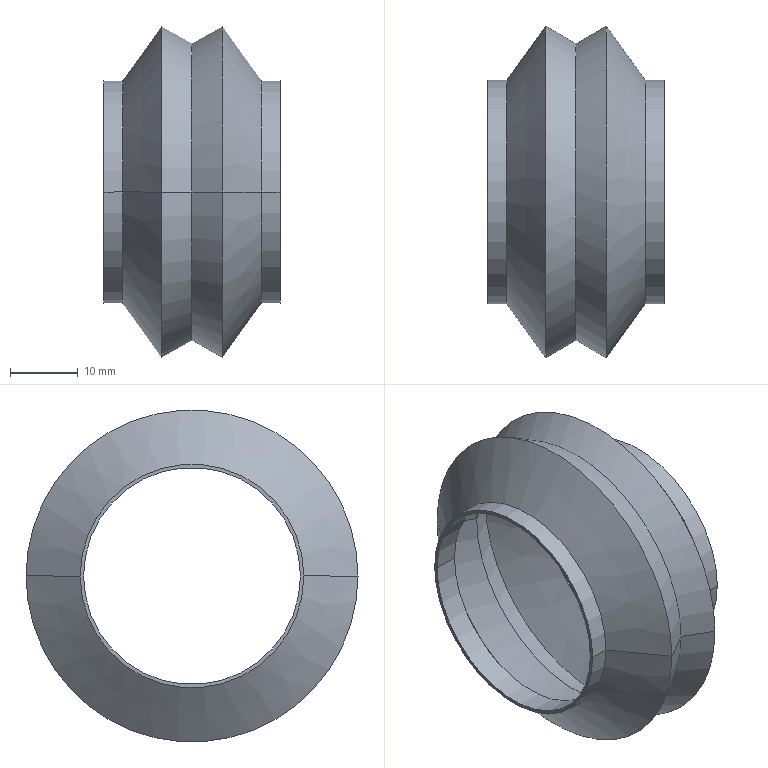Part | SolidWorks | features ICE 1, RevCut 1, Revolution 1 | 1 solid | 26 faces | box 26 x 49 x 49 mm | volume 4109 mm3 | cone 16 | cylinder 8 | plane 2 | commonest cylinder face diameters 32 x4 33 x4
STEP:
#1=CARTESIAN_POINT('',(-9.378,16.,0.));
#2=VERTEX_POINT('',#1);
#3=CARTESIAN_POINT('',(-9.378,-16.,0.));
#4=VERTEX_POINT('',#3);
#5=CARTESIAN_POINT('',(-9.378,0.,0.));
#6=DIRECTION('',(-1.,0.,0.));
#7=DIRECTION('',(0.,1.,0.));
#8=AXIS2_PLACEMENT_3D('',#5,#6,#7);
#9=CIRCLE('',#8,16.);
#10=EDGE_CURVE('',#2,#4,#9,.T.);
#11=ORIENTED_EDGE('',*,*,#10,.T.);
#12=CARTESIAN_POINT('',(-4.216,-23.181,0.));
#13=VERTEX_POINT('',#12);
#14=CARTESIAN_POINT('',(-4.216,-23.181,0.));
#15=DIRECTION('',(0.5836,-0.812,0.));
#16=VECTOR('',#15,1000.);
#17=LINE('',#14,#16);
#18=EDGE_CURVE('',#4,#13,#17,.T.);
#19=ORIENTED_EDGE('',*,*,#18,.T.);
#20=CARTESIAN_POINT('',(-4.216,23.181,0.));
#21=VERTEX_POINT('',#20);
#22=CARTESIAN_POINT('',(-4.216,0.,0.));
#23=DIRECTION('',(1.,0.,0.));
#24=DIRECTION('',(0.,1.,0.));
#25=AXIS2_PLACEMENT_3D('',#22,#23,#24);
#26=CIRCLE('',#25,23.181);
#27=EDGE_CURVE('',#13,#21,#26,.T.);
#28=ORIENTED_EDGE('',*,*,#27,.T.);
#29=CARTESIAN_POINT('',(-4.216,23.181,0.));
#30=DIRECTION('',(0.5836,0.812,0.));
#31=VECTOR('',#30,1000.);
#32=LINE('',#29,#31);
#33=EDGE_CURVE('',#2,#21,#32,.T.);
#34=ORIENTED_EDGE('',*,*,#33,.F.);
#35=EDGE_LOOP('',(#11,#19,#28,#34));
#36=FACE_OUTER_BOUND('',#35,.T.);
#37=CARTESIAN_POINT('',(-4.216,0.,0.));
#38=DIRECTION('',(1.,0.,0.));
#39=DIRECTION('',(0.,1.,0.));
#40=AXIS2_PLACEMENT_3D('',#37,#38,#39);
#41=CONICAL_SURFACE('',#40,23.181,0.9476);
#42=ADVANCED_FACE('',(#36),#41,.F.);
#43=CARTESIAN_POINT('',(0.,-20.747,0.));
#44=VERTEX_POINT('',#43);
#45=CARTESIAN_POINT('',(0.,20.747,0.));
#46=VERTEX_POINT('',#45);
#47=CARTESIAN_POINT('',(0.,0.,0.));
#48=DIRECTION('',(1.,0.,0.));
#49=DIRECTION('',(0.,1.,0.));
#50=AXIS2_PLACEMENT_3D('',#47,#48,#49);
#51=CIRCLE('',#50,20.747);
#52=EDGE_CURVE('',#44,#46,#51,.T.);
#53=ORIENTED_EDGE('',*,*,#52,.T.);
#54=CARTESIAN_POINT('',(0.,20.747,0.));
#55=DIRECTION('',(-0.866,0.5,0.));
#56=VECTOR('',#55,1000.);
#57=LINE('',#54,#56);
#58=EDGE_CURVE('',#46,#21,#57,.T.);
#59=ORIENTED_EDGE('',*,*,#58,.T.);
#60=ORIENTED_EDGE('',*,*,#27,.F.);
#61=CARTESIAN_POINT('',(0.,-20.747,0.));
#62=DIRECTION('',(-0.866,-0.5,0.));
#63=VECTOR('',#62,1000.);
#64=LINE('',#61,#63);
#65=EDGE_CURVE('',#44,#13,#64,.T.);
#66=ORIENTED_EDGE('',*,*,#65,.F.);
#67=EDGE_LOOP('',(#53,#59,#60,#66));
#68=FACE_OUTER_BOUND('',#67,.T.);
#69=CARTESIAN_POINT('',(0.,0.,0.));
#70=DIRECTION('',(-1.,0.,0.));
#71=DIRECTION('',(0.,-1.,0.));
#72=AXIS2_PLACEMENT_3D('',#69,#70,#71);
#73=CONICAL_SURFACE('',#72,20.747,0.5236);
#74=ADVANCED_FACE('',(#68),#73,.F.);
#75=ORIENTED_EDGE('',*,*,#52,.F.);
#76=CARTESIAN_POINT('',(4.216,-23.181,0.));
#77=VERTEX_POINT('',#76);
#78=CARTESIAN_POINT('',(4.216,-23.181,0.));
#79=DIRECTION('',(0.866,-0.5,0.));
#80=VECTOR('',#79,1000.);
#81=LINE('',#78,#80);
#82=EDGE_CURVE('',#44,#77,#81,.T.);
#83=ORIENTED_EDGE('',*,*,#82,.T.);
#84=CARTESIAN_POINT('',(4.216,23.181,0.));
#85=VERTEX_POINT('',#84);
#86=CARTESIAN_POINT('',(4.216,0.,0.));
#87=DIRECTION('',(1.,0.,0.));
#88=DIRECTION('',(0.,1.,0.));
#89=AXIS2_PLACEMENT_3D('',#86,#87,#88);
#90=CIRCLE('',#89,23.181);
#91=EDGE_CURVE('',#77,#85,#90,.T.);
#92=ORIENTED_EDGE('',*,*,#91,.T.);
#93=CARTESIAN_POINT('',(4.216,23.181,0.));
#94=DIRECTION('',(0.866,0.5,0.));
#95=VECTOR('',#94,1000.);
#96=LINE('',#93,#95);
#97=EDGE_CURVE('',#46,#85,#96,.T.);
#98=ORIENTED_EDGE('',*,*,#97,.F.);
#99=EDGE_LOOP('',(#75,#83,#92,#98));
#100=FACE_OUTER_BOUND('',#99,.T.);
#101=CARTESIAN_POINT('',(4.216,0.,0.));
#102=DIRECTION('',(1.,0.,0.));
#103=DIRECTION('',(0.,1.,0.));
#104=AXIS2_PLACEMENT_3D('',#101,#102,#103);
#105=CONICAL_SURFACE('',#104,23.181,0.5236);
#106=ADVANCED_FACE('',(#100),#105,.F.);
#107=CARTESIAN_POINT('',(9.378,-16.,0.));
#108=VERTEX_POINT('',#107);
#109=CARTESIAN_POINT('',(9.378,16.,0.));
#110=VERTEX_POINT('',#109);
#111=CARTESIAN_POINT('',(9.378,0.,0.));
#112=DIRECTION('',(1.,0.,0.));
#113=DIRECTION('',(0.,-1.,0.));
#114=AXIS2_PLACEMENT_3D('',#111,#112,#113);
#115=CIRCLE('',#114,16.);
#116=EDGE_CURVE('',#108,#110,#115,.T.);
#117=ORIENTED_EDGE('',*,*,#116,.T.);
#118=CARTESIAN_POINT('',(9.737,15.5,0.));
#119=DIRECTION('',(-0.5836,0.812,0.));
#120=VECTOR('',#119,1000.);
#121=LINE('',#118,#120);
#122=EDGE_CURVE('',#110,#85,#121,.T.);
#123=ORIENTED_EDGE('',*,*,#122,.T.);
#124=ORIENTED_EDGE('',*,*,#91,.F.);
#125=CARTESIAN_POINT('',(9.737,-15.5,0.));
#126=DIRECTION('',(-0.5836,-0.812,0.));
#127=VECTOR('',#126,1000.);
#128=LINE('',#125,#127);
#129=EDGE_CURVE('',#108,#77,#128,.T.);
#130=ORIENTED_EDGE('',*,*,#129,.F.);
#131=EDGE_LOOP('',(#117,#123,#124,#130));
#132=FACE_OUTER_BOUND('',#131,.T.);
#133=CARTESIAN_POINT('',(9.737,0.,0.));
#134=DIRECTION('',(-1.,0.,0.));
#135=DIRECTION('',(0.,-1.,0.));
#136=AXIS2_PLACEMENT_3D('',#133,#134,#135);
#137=CONICAL_SURFACE('',#136,15.5,0.9476);
#138=ADVANCED_FACE('',(#132),#137,.F.);
#139=ORIENTED_EDGE('',*,*,#116,.F.);
#140=CARTESIAN_POINT('',(13.,-16.,0.));
#141=VERTEX_POINT('',#140);
#142=CARTESIAN_POINT('',(-107.,-16.,0.));
#143=DIRECTION('',(1.,0.,0.));
#144=VECTOR('',#143,1000.);
#145=LINE('',#142,#144);
#146=EDGE_CURVE('',#108,#141,#145,.T.);
#147=ORIENTED_EDGE('',*,*,#146,.T.);
#148=CARTESIAN_POINT('',(13.,16.,0.));
#149=VERTEX_POINT('',#148);
#150=CARTESIAN_POINT('',(13.,0.,0.));
#151=DIRECTION('',(1.,0.,0.));
#152=DIRECTION('',(0.,1.,0.));
#153=AXIS2_PLACEMENT_3D('',#150,#151,#152);
#154=CIRCLE('',#153,16.);
#155=EDGE_CURVE('',#141,#149,#154,.T.);
#156=ORIENTED_EDGE('',*,*,#155,.T.);
#157=CARTESIAN_POINT('',(-107.,16.,0.));
#158=DIRECTION('',(1.,0.,0.));
#159=VECTOR('',#158,1000.);
#160=LINE('',#157,#159);
#161=EDGE_CURVE('',#110,#149,#160,.T.);
#162=ORIENTED_EDGE('',*,*,#161,.F.);
#163=EDGE_LOOP('',(#139,#147,#156,#162));
#164=FACE_OUTER_BOUND('',#163,.T.);
#165=CARTESIAN_POINT('',(-107.,0.,0.));
#166=DIRECTION('',(1.,0.,0.));
#167=DIRECTION('',(0.,1.,0.));
#168=AXIS2_PLACEMENT_3D('',#165,#166,#167);
#169=CYLINDRICAL_SURFACE('',#168,16.);
#170=ADVANCED_FACE('',(#164),#169,.F.);
#171=CARTESIAN_POINT('',(-13.,-16.,0.));
#172=VERTEX_POINT('',#171);
#173=CARTESIAN_POINT('',(-13.,16.,0.));
#174=VERTEX_POINT('',#173);
#175=CARTESIAN_POINT('',(-13.,0.,0.));
#176=DIRECTION('',(1.,0.,0.));
#177=DIRECTION('',(0.,1.,0.));
#178=AXIS2_PLACEMENT_3D('',#175,#176,#177);
#179=CIRCLE('',#178,16.);
#180=EDGE_CURVE('',#172,#174,#179,.T.);
#181=ORIENTED_EDGE('',*,*,#180,.F.);
#182=CARTESIAN_POINT('',(-107.,-16.,0.));
#183=DIRECTION('',(1.,0.,0.));
#184=VECTOR('',#183,1000.);
#185=LINE('',#182,#184);
#186=EDGE_CURVE('',#172,#4,#185,.T.);
#187=ORIENTED_EDGE('',*,*,#186,.T.);
#188=ORIENTED_EDGE('',*,*,#10,.F.);
#189=CARTESIAN_POINT('',(-107.,16.,0.));
#190=DIRECTION('',(1.,0.,0.));
#191=VECTOR('',#190,1000.);
#192=LINE('',#189,#191);
#193=EDGE_CURVE('',#174,#2,#192,.T.);
#194=ORIENTED_EDGE('',*,*,#193,.F.);
#195=EDGE_LOOP('',(#181,#187,#188,#194));
#196=FACE_OUTER_BOUND('',#195,.T.);
#197=CARTESIAN_POINT('',(-107.,0.,0.));
#198=DIRECTION('',(1.,0.,0.));
#199=DIRECTION('',(0.,1.,0.));
#200=AXIS2_PLACEMENT_3D('',#197,#198,#199);
#201=CYLINDRICAL_SURFACE('',#200,16.);
#202=ADVANCED_FACE('',(#196),#201,.F.);
#203=CARTESIAN_POINT('',(0.,-21.902,0.));
#204=VERTEX_POINT('',#203);
#205=CARTESIAN_POINT('',(0.,21.902,0.));
#206=VERTEX_POINT('',#205);
#207=CARTESIAN_POINT('',(0.,0.,0.));
#208=DIRECTION('',(-1.,0.,0.));
#209=DIRECTION('',(0.,-1.,0.));
#210=AXIS2_PLACEMENT_3D('',#207,#208,#209);
#211=CIRCLE('',#210,21.902);
#212=EDGE_CURVE('',#204,#206,#211,.T.);
#213=ORIENTED_EDGE('',*,*,#212,.F.);
#214=CARTESIAN_POINT('',(4.5,-24.5,0.));
#215=VERTEX_POINT('',#214);
#216=CARTESIAN_POINT('',(4.5,-24.5,0.));
#217=DIRECTION('',(0.866,-0.5,0.));
#218=VECTOR('',#217,1000.);
#219=LINE('',#216,#218);
#220=EDGE_CURVE('',#204,#215,#219,.T.);
#221=ORIENTED_EDGE('',*,*,#220,.T.);
#222=CARTESIAN_POINT('',(4.5,24.5,0.));
#223=VERTEX_POINT('',#222);
#224=CARTESIAN_POINT('',(4.5,0.,0.));
#225=DIRECTION('',(-1.,0.,0.));
#226=DIRECTION('',(0.,-1.,0.));
#227=AXIS2_PLACEMENT_3D('',#224,#225,#226);
#228=CIRCLE('',#227,24.5);
#229=EDGE_CURVE('',#215,#223,#228,.T.);
#230=ORIENTED_EDGE('',*,*,#229,.T.);
#231=CARTESIAN_POINT('',(4.5,24.5,0.));
#232=DIRECTION('',(0.866,0.5,0.));
#233=VECTOR('',#232,1000.);
#234=LINE('',#231,#233);
#235=EDGE_CURVE('',#206,#223,#234,.T.);
#236=ORIENTED_EDGE('',*,*,#235,.F.);
#237=EDGE_LOOP('',(#213,#221,#230,#236));
#238=FACE_OUTER_BOUND('',#237,.T.);
#239=CARTESIAN_POINT('',(4.5,0.,0.));
#240=DIRECTION('',(1.,0.,0.));
#241=DIRECTION('',(0.,1.,0.));
#242=AXIS2_PLACEMENT_3D('',#239,#240,#241);
#243=CONICAL_SURFACE('',#242,24.5,0.5236);
#244=ADVANCED_FACE('',(#238),#243,.T.);
#245=CARTESIAN_POINT('',(10.25,-16.5,0.));
#246=VERTEX_POINT('',#245);
#247=CARTESIAN_POINT('',(10.25,16.5,0.));
#248=VERTEX_POINT('',#247);
#249=CARTESIAN_POINT('',(10.25,0.,0.));
#250=DIRECTION('',(-1.,0.,0.));
#251=DIRECTION('',(0.,-1.,0.));
#252=AXIS2_PLACEMENT_3D('',#249,#250,#251);
#253=CIRCLE('',#252,16.5);
#254=EDGE_CURVE('',#246,#248,#253,.T.);
#255=ORIENTED_EDGE('',*,*,#254,.T.);
#256=CARTESIAN_POINT('',(10.25,16.5,0.));
#257=DIRECTION('',(-0.5836,0.812,0.));
#258=VECTOR('',#257,1000.);
#259=LINE('',#256,#258);
#260=EDGE_CURVE('',#248,#223,#259,.T.);
#261=ORIENTED_EDGE('',*,*,#260,.T.);
#262=ORIENTED_EDGE('',*,*,#229,.F.);
#263=CARTESIAN_POINT('',(10.25,-16.5,0.));
#264=DIRECTION('',(-0.5836,-0.812,0.));
#265=VECTOR('',#264,1000.);
#266=LINE('',#263,#265);
#267=EDGE_CURVE('',#246,#215,#266,.T.);
#268=ORIENTED_EDGE('',*,*,#267,.F.);
#269=EDGE_LOOP('',(#255,#261,#262,#268));
#270=FACE_OUTER_BOUND('',#269,.T.);
#271=CARTESIAN_POINT('',(10.25,0.,0.));
#272=DIRECTION('',(-1.,0.,0.));
#273=DIRECTION('',(0.,-1.,0.));
#274=AXIS2_PLACEMENT_3D('',#271,#272,#273);
#275=CONICAL_SURFACE('',#274,16.5,0.9476);
#276=ADVANCED_FACE('',(#270),#275,.T.);
#277=CARTESIAN_POINT('',(13.,-16.5,0.));
#278=VERTEX_POINT('',#277);
#279=CARTESIAN_POINT('',(13.,16.5,0.));
#280=VERTEX_POINT('',#279);
#281=CARTESIAN_POINT('',(13.,0.,0.));
#282=DIRECTION('',(-1.,0.,0.));
#283=DIRECTION('',(0.,-1.,0.));
#284=AXIS2_PLACEMENT_3D('',#281,#282,#283);
#285=CIRCLE('',#284,16.5);
#286=EDGE_CURVE('',#278,#280,#285,.T.);
#287=ORIENTED_EDGE('',*,*,#286,.T.);
#288=CARTESIAN_POINT('',(-38.098,16.5,0.));
#289=DIRECTION('',(-1.,0.,0.));
#290=VECTOR('',#289,1000.);
#291=LINE('',#288,#290);
#292=EDGE_CURVE('',#280,#248,#291,.T.);
#293=ORIENTED_EDGE('',*,*,#292,.T.);
#294=ORIENTED_EDGE('',*,*,#254,.F.);
#295=CARTESIAN_POINT('',(-38.098,-16.5,0.));
#296=DIRECTION('',(-1.,0.,0.));
#297=VECTOR('',#296,1000.);
#298=LINE('',#295,#297);
#299=EDGE_CURVE('',#278,#246,#298,.T.);
#300=ORIENTED_EDGE('',*,*,#299,.F.);
#301=EDGE_LOOP('',(#287,#293,#294,#300));
#302=FACE_OUTER_BOUND('',#301,.T.);
#303=CARTESIAN_POINT('',(-38.098,0.,0.));
#304=DIRECTION('',(-1.,0.,0.));
#305=DIRECTION('',(0.,-1.,0.));
#306=AXIS2_PLACEMENT_3D('',#303,#304,#305);
#307=CYLINDRICAL_SURFACE('',#306,16.5);
#308=ADVANCED_FACE('',(#302),#307,.T.);
#309=CARTESIAN_POINT('',(-10.25,-16.5,0.));
#310=VERTEX_POINT('',#309);
#311=CARTESIAN_POINT('',(-10.25,16.5,0.));
#312=VERTEX_POINT('',#311);
#313=CARTESIAN_POINT('',(-10.25,0.,0.));
#314=DIRECTION('',(-1.,0.,0.));
#315=DIRECTION('',(0.,-1.,0.));
#316=AXIS2_PLACEMENT_3D('',#313,#314,#315);
#317=CIRCLE('',#316,16.5);
#318=EDGE_CURVE('',#310,#312,#317,.T.);
#319=ORIENTED_EDGE('',*,*,#318,.T.);
#320=CARTESIAN_POINT('',(-13.,16.5,0.));
#321=VERTEX_POINT('',#320);
#322=CARTESIAN_POINT('',(-38.098,16.5,0.));
#323=DIRECTION('',(-1.,0.,0.));
#324=VECTOR('',#323,1000.);
#325=LINE('',#322,#324);
#326=EDGE_CURVE('',#312,#321,#325,.T.);
#327=ORIENTED_EDGE('',*,*,#326,.T.);
#328=CARTESIAN_POINT('',(-13.,-16.5,0.));
#329=VERTEX_POINT('',#328);
#330=CARTESIAN_POINT('',(-13.,0.,0.));
#331=DIRECTION('',(-1.,0.,0.));
#332=DIRECTION('',(0.,-1.,0.));
#333=AXIS2_PLACEMENT_3D('',#330,#331,#332);
#334=CIRCLE('',#333,16.5);
#335=EDGE_CURVE('',#329,#321,#334,.T.);
#336=ORIENTED_EDGE('',*,*,#335,.F.);
#337=CARTESIAN_POINT('',(-38.098,-16.5,0.));
#338=DIRECTION('',(-1.,0.,0.));
#339=VECTOR('',#338,1000.);
#340=LINE('',#337,#339);
#341=EDGE_CURVE('',#310,#329,#340,.T.);
#342=ORIENTED_EDGE('',*,*,#341,.F.);
#343=EDGE_LOOP('',(#319,#327,#336,#342));
#344=FACE_OUTER_BOUND('',#343,.T.);
#345=CARTESIAN_POINT('',(-38.098,0.,0.));
#346=DIRECTION('',(-1.,0.,0.));
#347=DIRECTION('',(0.,-1.,0.));
#348=AXIS2_PLACEMENT_3D('',#345,#346,#347);
#349=CYLINDRICAL_SURFACE('',#348,16.5);
#350=ADVANCED_FACE('',(#344),#349,.T.);
#351=ORIENTED_EDGE('',*,*,#318,.F.);
#352=CARTESIAN_POINT('',(-4.5,-24.5,0.));
#353=VERTEX_POINT('',#352);
#354=CARTESIAN_POINT('',(-4.5,-24.5,0.));
#355=DIRECTION('',(0.5836,-0.812,0.));
#356=VECTOR('',#355,1000.);
#357=LINE('',#354,#356);
#358=EDGE_CURVE('',#310,#353,#357,.T.);
#359=ORIENTED_EDGE('',*,*,#358,.T.);
#360=CARTESIAN_POINT('',(-4.5,24.5,0.));
#361=VERTEX_POINT('',#360);
#362=CARTESIAN_POINT('',(-4.5,0.,0.));
#363=DIRECTION('',(-1.,0.,0.));
#364=DIRECTION('',(0.,-1.,0.));
#365=AXIS2_PLACEMENT_3D('',#362,#363,#364);
#366=CIRCLE('',#365,24.5);
#367=EDGE_CURVE('',#353,#361,#366,.T.);
#368=ORIENTED_EDGE('',*,*,#367,.T.);
#369=CARTESIAN_POINT('',(-4.5,24.5,0.));
#370=DIRECTION('',(0.5836,0.812,0.));
#371=VECTOR('',#370,1000.);
#372=LINE('',#369,#371);
#373=EDGE_CURVE('',#312,#361,#372,.T.);
#374=ORIENTED_EDGE('',*,*,#373,.F.);
#375=EDGE_LOOP('',(#351,#359,#368,#374));
#376=FACE_OUTER_BOUND('',#375,.T.);
#377=CARTESIAN_POINT('',(-4.5,0.,0.));
#378=DIRECTION('',(1.,0.,0.));
#379=DIRECTION('',(0.,1.,0.));
#380=AXIS2_PLACEMENT_3D('',#377,#378,#379);
#381=CONICAL_SURFACE('',#380,24.5,0.9476);
#382=ADVANCED_FACE('',(#376),#381,.T.);
#383=ORIENTED_EDGE('',*,*,#212,.T.);
#384=CARTESIAN_POINT('',(0.,21.902,0.));
#385=DIRECTION('',(-0.866,0.5,0.));
#386=VECTOR('',#385,1000.);
#387=LINE('',#384,#386);
#388=EDGE_CURVE('',#206,#361,#387,.T.);
#389=ORIENTED_EDGE('',*,*,#388,.T.);
#390=ORIENTED_EDGE('',*,*,#367,.F.);
#391=CARTESIAN_POINT('',(0.,-21.902,0.));
#392=DIRECTION('',(-0.866,-0.5,0.));
#393=VECTOR('',#392,1000.);
#394=LINE('',#391,#393);
#395=EDGE_CURVE('',#204,#353,#394,.T.);
#396=ORIENTED_EDGE('',*,*,#395,.F.);
#397=EDGE_LOOP('',(#383,#389,#390,#396));
#398=FACE_OUTER_BOUND('',#397,.T.);
#399=CARTESIAN_POINT('',(0.,0.,0.));
#400=DIRECTION('',(-1.,0.,0.));
#401=DIRECTION('',(0.,-1.,0.));
#402=AXIS2_PLACEMENT_3D('',#399,#400,#401);
#403=CONICAL_SURFACE('',#402,21.902,0.5236);
#404=ADVANCED_FACE('',(#398),#403,.T.);
#405=ORIENTED_EDGE('',*,*,#388,.F.);
#406=CARTESIAN_POINT('',(0.,0.,0.));
#407=DIRECTION('',(-1.,0.,0.));
#408=DIRECTION('',(0.,-1.,0.));
#409=AXIS2_PLACEMENT_3D('',#406,#407,#408);
#410=CIRCLE('',#409,21.902);
#411=EDGE_CURVE('',#206,#204,#410,.T.);
#412=ORIENTED_EDGE('',*,*,#411,.T.);
#413=ORIENTED_EDGE('',*,*,#395,.T.);
#414=CARTESIAN_POINT('',(-4.5,0.,0.));
#415=DIRECTION('',(-1.,0.,0.));
#416=DIRECTION('',(0.,-1.,0.));
#417=AXIS2_PLACEMENT_3D('',#414,#415,#416);
#418=CIRCLE('',#417,24.5);
#419=EDGE_CURVE('',#361,#353,#418,.T.);
#420=ORIENTED_EDGE('',*,*,#419,.F.);
#421=EDGE_LOOP('',(#405,#412,#413,#420));
#422=FACE_OUTER_BOUND('',#421,.T.);
#423=CARTESIAN_POINT('',(0.,0.,0.));
#424=DIRECTION('',(-1.,0.,0.));
#425=DIRECTION('',(0.,-1.,0.));
#426=AXIS2_PLACEMENT_3D('',#423,#424,#425);
#427=CONICAL_SURFACE('',#426,21.902,0.5236);
#428=ADVANCED_FACE('',(#422),#427,.T.);
#429=ORIENTED_EDGE('',*,*,#358,.F.);
#430=CARTESIAN_POINT('',(-10.25,0.,0.));
#431=DIRECTION('',(-1.,0.,0.));
#432=DIRECTION('',(0.,-1.,0.));
#433=AXIS2_PLACEMENT_3D('',#430,#431,#432);
#434=CIRCLE('',#433,16.5);
#435=EDGE_CURVE('',#312,#310,#434,.T.);
#436=ORIENTED_EDGE('',*,*,#435,.F.);
#437=ORIENTED_EDGE('',*,*,#373,.T.);
#438=ORIENTED_EDGE('',*,*,#419,.T.);
#439=EDGE_LOOP('',(#429,#436,#437,#438));
#440=FACE_OUTER_BOUND('',#439,.T.);
#441=CARTESIAN_POINT('',(-4.5,0.,0.));
#442=DIRECTION('',(1.,0.,0.));
#443=DIRECTION('',(0.,1.,0.));
#444=AXIS2_PLACEMENT_3D('',#441,#442,#443);
#445=CONICAL_SURFACE('',#444,24.5,0.9476);
#446=ADVANCED_FACE('',(#440),#445,.T.);
#447=ORIENTED_EDGE('',*,*,#326,.F.);
#448=ORIENTED_EDGE('',*,*,#435,.T.);
#449=ORIENTED_EDGE('',*,*,#341,.T.);
#450=CARTESIAN_POINT('',(-13.,0.,0.));
#451=DIRECTION('',(-1.,0.,0.));
#452=DIRECTION('',(0.,-1.,0.));
#453=AXIS2_PLACEMENT_3D('',#450,#451,#452);
#454=CIRCLE('',#453,16.5);
#455=EDGE_CURVE('',#321,#329,#454,.T.);
#456=ORIENTED_EDGE('',*,*,#455,.F.);
#457=EDGE_LOOP('',(#447,#448,#449,#456));
#458=FACE_OUTER_BOUND('',#457,.T.);
#459=CARTESIAN_POINT('',(-38.098,0.,0.));
#460=DIRECTION('',(-1.,0.,0.));
#461=DIRECTION('',(0.,-1.,0.));
#462=AXIS2_PLACEMENT_3D('',#459,#460,#461);
#463=CYLINDRICAL_SURFACE('',#462,16.5);
#464=ADVANCED_FACE('',(#458),#463,.T.);
#465=CARTESIAN_POINT('',(-13.,0.,0.));
#466=DIRECTION('',(1.,0.,0.));
#467=DIRECTION('',(0.,1.,0.));
#468=AXIS2_PLACEMENT_3D('',#465,#466,#467);
#469=CIRCLE('',#468,16.);
#470=EDGE_CURVE('',#174,#172,#469,.T.);
#471=ORIENTED_EDGE('',*,*,#470,.T.);
#472=ORIENTED_EDGE('',*,*,#180,.T.);
#473=EDGE_LOOP('',(#471,#472));
#474=FACE_BOUND('',#473,.T.);
#475=ORIENTED_EDGE('',*,*,#335,.T.);
#476=ORIENTED_EDGE('',*,*,#455,.T.);
#477=EDGE_LOOP('',(#475,#476));
#478=FACE_OUTER_BOUND('',#477,.T.);
#479=CARTESIAN_POINT('',(-13.,16.5,0.));
#480=DIRECTION('',(1.,0.,0.));
#481=DIRECTION('',(0.,1.,0.));
#482=AXIS2_PLACEMENT_3D('',#479,#480,#481);
#483=PLANE('',#482);
#484=ADVANCED_FACE('',(#474,#478),#483,.F.);
#485=CARTESIAN_POINT('',(13.,0.,0.));
#486=DIRECTION('',(1.,0.,0.));
#487=DIRECTION('',(0.,1.,0.));
#488=AXIS2_PLACEMENT_3D('',#485,#486,#487);
#489=CIRCLE('',#488,16.);
#490=EDGE_CURVE('',#149,#141,#489,.T.);
#491=ORIENTED_EDGE('',*,*,#490,.F.);
#492=ORIENTED_EDGE('',*,*,#155,.F.);
#493=EDGE_LOOP('',(#491,#492));
#494=FACE_BOUND('',#493,.T.);
#495=ORIENTED_EDGE('',*,*,#286,.F.);
#496=CARTESIAN_POINT('',(13.,0.,0.));
#497=DIRECTION('',(-1.,0.,0.));
#498=DIRECTION('',(0.,-1.,0.));
#499=AXIS2_PLACEMENT_3D('',#496,#497,#498);
#500=CIRCLE('',#499,16.5);
#501=EDGE_CURVE('',#280,#278,#500,.T.);
#502=ORIENTED_EDGE('',*,*,#501,.F.);
#503=EDGE_LOOP('',(#495,#502));
#504=FACE_OUTER_BOUND('',#503,.T.);
#505=CARTESIAN_POINT('',(13.,16.5,0.));
#506=DIRECTION('',(-1.,0.,0.));
#507=DIRECTION('',(0.,-1.,0.));
#508=AXIS2_PLACEMENT_3D('',#505,#506,#507);
#509=PLANE('',#508);
#510=ADVANCED_FACE('',(#494,#504),#509,.F.);
#511=ORIENTED_EDGE('',*,*,#292,.F.);
#512=ORIENTED_EDGE('',*,*,#501,.T.);
#513=ORIENTED_EDGE('',*,*,#299,.T.);
#514=CARTESIAN_POINT('',(10.25,0.,0.));
#515=DIRECTION('',(-1.,0.,0.));
#516=DIRECTION('',(0.,-1.,0.));
#517=AXIS2_PLACEMENT_3D('',#514,#515,#516);
#518=CIRCLE('',#517,16.5);
#519=EDGE_CURVE('',#248,#246,#518,.T.);
#520=ORIENTED_EDGE('',*,*,#519,.F.);
#521=EDGE_LOOP('',(#511,#512,#513,#520));
#522=FACE_OUTER_BOUND('',#521,.T.);
#523=CARTESIAN_POINT('',(-38.098,0.,0.));
#524=DIRECTION('',(-1.,0.,0.));
#525=DIRECTION('',(0.,-1.,0.));
#526=AXIS2_PLACEMENT_3D('',#523,#524,#525);
#527=CYLINDRICAL_SURFACE('',#526,16.5);
#528=ADVANCED_FACE('',(#522),#527,.T.);
#529=ORIENTED_EDGE('',*,*,#260,.F.);
#530=ORIENTED_EDGE('',*,*,#519,.T.);
#531=ORIENTED_EDGE('',*,*,#267,.T.);
#532=CARTESIAN_POINT('',(4.5,0.,0.));
#533=DIRECTION('',(-1.,0.,0.));
#534=DIRECTION('',(0.,-1.,0.));
#535=AXIS2_PLACEMENT_3D('',#532,#533,#534);
#536=CIRCLE('',#535,24.5);
#537=EDGE_CURVE('',#223,#215,#536,.T.);
#538=ORIENTED_EDGE('',*,*,#537,.F.);
#539=EDGE_LOOP('',(#529,#530,#531,#538));
#540=FACE_OUTER_BOUND('',#539,.T.);
#541=CARTESIAN_POINT('',(10.25,0.,0.));
#542=DIRECTION('',(-1.,0.,0.));
#543=DIRECTION('',(0.,-1.,0.));
#544=AXIS2_PLACEMENT_3D('',#541,#542,#543);
#545=CONICAL_SURFACE('',#544,16.5,0.9476);
#546=ADVANCED_FACE('',(#540),#545,.T.);
#547=ORIENTED_EDGE('',*,*,#220,.F.);
#548=ORIENTED_EDGE('',*,*,#411,.F.);
#549=ORIENTED_EDGE('',*,*,#235,.T.);
#550=ORIENTED_EDGE('',*,*,#537,.T.);
#551=EDGE_LOOP('',(#547,#548,#549,#550));
#552=FACE_OUTER_BOUND('',#551,.T.);
#553=CARTESIAN_POINT('',(4.5,0.,0.));
#554=DIRECTION('',(1.,0.,0.));
#555=DIRECTION('',(0.,1.,0.));
#556=AXIS2_PLACEMENT_3D('',#553,#554,#555);
#557=CONICAL_SURFACE('',#556,24.5,0.5236);
#558=ADVANCED_FACE('',(#552),#557,.T.);
#559=ORIENTED_EDGE('',*,*,#186,.F.);
#560=ORIENTED_EDGE('',*,*,#470,.F.);
#561=ORIENTED_EDGE('',*,*,#193,.T.);
#562=CARTESIAN_POINT('',(-9.378,0.,0.));
#563=DIRECTION('',(-1.,0.,0.));
#564=DIRECTION('',(0.,1.,0.));
#565=AXIS2_PLACEMENT_3D('',#562,#563,#564);
#566=CIRCLE('',#565,16.);
#567=EDGE_CURVE('',#4,#2,#566,.T.);
#568=ORIENTED_EDGE('',*,*,#567,.F.);
#569=EDGE_LOOP('',(#559,#560,#561,#568));
#570=FACE_OUTER_BOUND('',#569,.T.);
#571=CARTESIAN_POINT('',(-107.,0.,0.));
#572=DIRECTION('',(1.,0.,0.));
#573=DIRECTION('',(0.,1.,0.));
#574=AXIS2_PLACEMENT_3D('',#571,#572,#573);
#575=CYLINDRICAL_SURFACE('',#574,16.);
#576=ADVANCED_FACE('',(#570),#575,.F.);
#577=ORIENTED_EDGE('',*,*,#146,.F.);
#578=CARTESIAN_POINT('',(9.378,0.,0.));
#579=DIRECTION('',(1.,0.,0.));
#580=DIRECTION('',(0.,-1.,0.));
#581=AXIS2_PLACEMENT_3D('',#578,#579,#580);
#582=CIRCLE('',#581,16.);
#583=EDGE_CURVE('',#110,#108,#582,.T.);
#584=ORIENTED_EDGE('',*,*,#583,.F.);
#585=ORIENTED_EDGE('',*,*,#161,.T.);
#586=ORIENTED_EDGE('',*,*,#490,.T.);
#587=EDGE_LOOP('',(#577,#584,#585,#586));
#588=FACE_OUTER_BOUND('',#587,.T.);
#589=CARTESIAN_POINT('',(-107.,0.,0.));
#590=DIRECTION('',(1.,0.,0.));
#591=DIRECTION('',(0.,1.,0.));
#592=AXIS2_PLACEMENT_3D('',#589,#590,#591);
#593=CYLINDRICAL_SURFACE('',#592,16.);
#594=ADVANCED_FACE('',(#588),#593,.F.);
#595=ORIENTED_EDGE('',*,*,#122,.F.);
#596=ORIENTED_EDGE('',*,*,#583,.T.);
#597=ORIENTED_EDGE('',*,*,#129,.T.);
#598=CARTESIAN_POINT('',(4.216,0.,0.));
#599=DIRECTION('',(1.,0.,0.));
#600=DIRECTION('',(0.,1.,0.));
#601=AXIS2_PLACEMENT_3D('',#598,#599,#600);
#602=CIRCLE('',#601,23.181);
#603=EDGE_CURVE('',#85,#77,#602,.T.);
#604=ORIENTED_EDGE('',*,*,#603,.F.);
#605=EDGE_LOOP('',(#595,#596,#597,#604));
#606=FACE_OUTER_BOUND('',#605,.T.);
#607=CARTESIAN_POINT('',(9.737,0.,0.));
#608=DIRECTION('',(-1.,0.,0.));
#609=DIRECTION('',(0.,-1.,0.));
#610=AXIS2_PLACEMENT_3D('',#607,#608,#609);
#611=CONICAL_SURFACE('',#610,15.5,0.9476);
#612=ADVANCED_FACE('',(#606),#611,.F.);
#613=ORIENTED_EDGE('',*,*,#82,.F.);
#614=CARTESIAN_POINT('',(0.,0.,0.));
#615=DIRECTION('',(1.,0.,0.));
#616=DIRECTION('',(0.,1.,0.));
#617=AXIS2_PLACEMENT_3D('',#614,#615,#616);
#618=CIRCLE('',#617,20.747);
#619=EDGE_CURVE('',#46,#44,#618,.T.);
#620=ORIENTED_EDGE('',*,*,#619,.F.);
#621=ORIENTED_EDGE('',*,*,#97,.T.);
#622=ORIENTED_EDGE('',*,*,#603,.T.);
#623=EDGE_LOOP('',(#613,#620,#621,#622));
#624=FACE_OUTER_BOUND('',#623,.T.);
#625=CARTESIAN_POINT('',(4.216,0.,0.));
#626=DIRECTION('',(1.,0.,0.));
#627=DIRECTION('',(0.,1.,0.));
#628=AXIS2_PLACEMENT_3D('',#625,#626,#627);
#629=CONICAL_SURFACE('',#628,23.181,0.5236);
#630=ADVANCED_FACE('',(#624),#629,.F.);
#631=ORIENTED_EDGE('',*,*,#58,.F.);
#632=ORIENTED_EDGE('',*,*,#619,.T.);
#633=ORIENTED_EDGE('',*,*,#65,.T.);
#634=CARTESIAN_POINT('',(-4.216,0.,0.));
#635=DIRECTION('',(1.,0.,0.));
#636=DIRECTION('',(0.,1.,0.));
#637=AXIS2_PLACEMENT_3D('',#634,#635,#636);
#638=CIRCLE('',#637,23.181);
#639=EDGE_CURVE('',#21,#13,#638,.T.);
#640=ORIENTED_EDGE('',*,*,#639,.F.);
#641=EDGE_LOOP('',(#631,#632,#633,#640));
#642=FACE_OUTER_BOUND('',#641,.T.);
#643=CARTESIAN_POINT('',(0.,0.,0.));
#644=DIRECTION('',(-1.,0.,0.));
#645=DIRECTION('',(0.,-1.,0.));
#646=AXIS2_PLACEMENT_3D('',#643,#644,#645);
#647=CONICAL_SURFACE('',#646,20.747,0.5236);
#648=ADVANCED_FACE('',(#642),#647,.F.);
#649=ORIENTED_EDGE('',*,*,#18,.F.);
#650=ORIENTED_EDGE('',*,*,#567,.T.);
#651=ORIENTED_EDGE('',*,*,#33,.T.);
#652=ORIENTED_EDGE('',*,*,#639,.T.);
#653=EDGE_LOOP('',(#649,#650,#651,#652));
#654=FACE_OUTER_BOUND('',#653,.T.);
#655=CARTESIAN_POINT('',(-4.216,0.,0.));
#656=DIRECTION('',(1.,0.,0.));
#657=DIRECTION('',(0.,1.,0.));
#658=AXIS2_PLACEMENT_3D('',#655,#656,#657);
#659=CONICAL_SURFACE('',#658,23.181,0.9476);
#660=ADVANCED_FACE('',(#654),#659,.F.);
#661=CLOSED_SHELL('',(#42,#74,#106,#138,#170,#202,#244,#276,#308,#350,#382,#404,#428,#446,#464,#484,#510,#528,#546,#558,#576,#594,#612,#630,#648,#660));
#662=MANIFOLD_SOLID_BREP('',#661);
#663=CARTESIAN_POINT('',(0.,0.,0.));
#664=DIRECTION('',(0.,0.,1.));
#665=DIRECTION('',(1.,0.,0.));
#666=AXIS2_PLACEMENT_3D('',#663,#664,#665);
#667=(LENGTH_UNIT()NAMED_UNIT(*)SI_UNIT(.MILLI.,.METRE.));
#668=UNCERTAINTY_MEASURE_WITH_UNIT(LENGTH_MEASURE(0.00001),#667,'','');
#669=(NAMED_UNIT(*)PLANE_ANGLE_UNIT()SI_UNIT($,.RADIAN.));
#670=(NAMED_UNIT(*)SI_UNIT($,.STERADIAN.)SOLID_ANGLE_UNIT());
#671=(GEOMETRIC_REPRESENTATION_CONTEXT(3)GLOBAL_UNCERTAINTY_ASSIGNED_CONTEXT((#668))GLOBAL_UNIT_ASSIGNED_CONTEXT((#667,#669,#670))REPRESENTATION_CONTEXT('',''));
#672=ADVANCED_BREP_SHAPE_REPRESENTATION('',(#662,#666),#671);